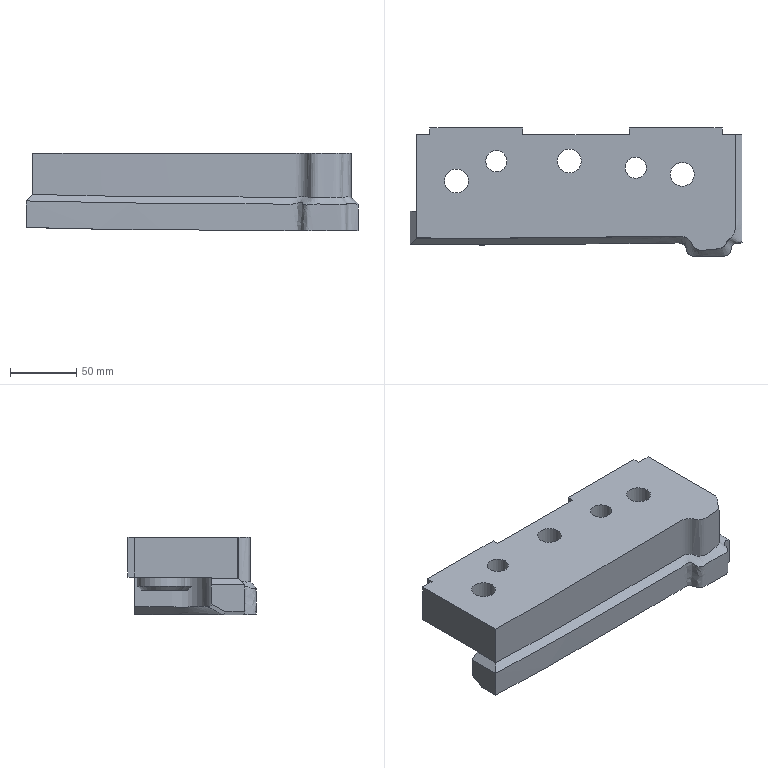Part | NX | features solid 2 | 1 solid | 38 faces | box 250 x 96.442 x 58.359 mm | volume 817854 mm3 | plane 20 | cylinder 10 | spline 6 | cone 2 | commonest cylinder face diameters 18 x3 26 x3 16 x2 36 x2